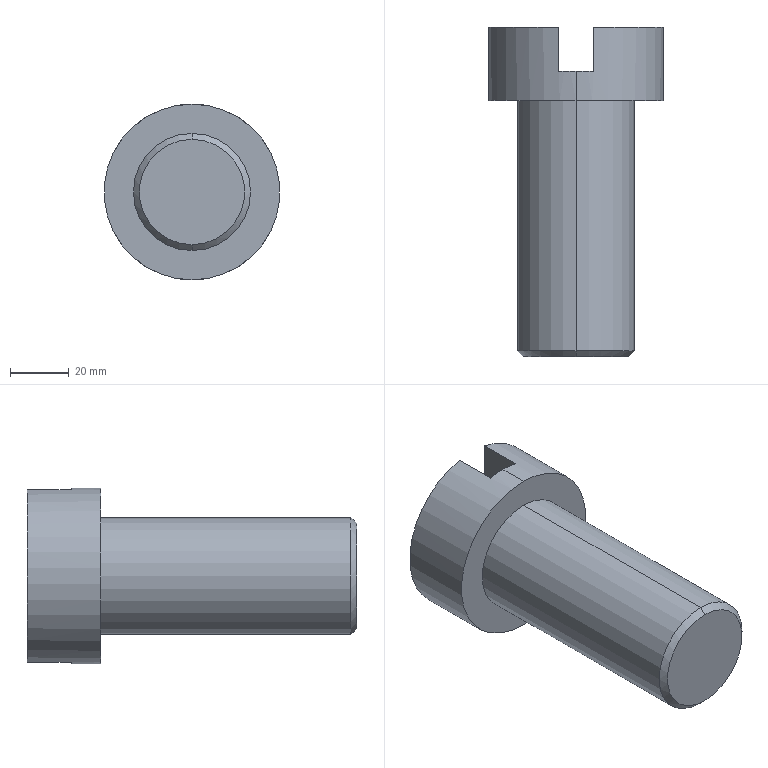Part | SolidWorks | features ICE 2, Chamfer 1, Extrusion 1 | 1 solid | 13 faces | box 60 x 112.5 x 60 mm | volume 169671 mm3 | plane 7 | cylinder 4 | cone 2 | commonest cylinder face diameters 40 x2 60 x2
STEP:
#1=CARTESIAN_POINT('',(0.,-50.,-18.));
#2=VERTEX_POINT('',#1);
#3=CARTESIAN_POINT('',(0.,-50.,18.));
#4=VERTEX_POINT('',#3);
#5=CARTESIAN_POINT('',(0.,-50.,0.));
#6=DIRECTION('',(0.,-1.,0.));
#7=DIRECTION('',(0.,0.,1.));
#8=AXIS2_PLACEMENT_3D('',#5,#6,#7);
#9=CIRCLE('',#8,18.);
#10=EDGE_CURVE('',#2,#4,#9,.T.);
#11=ORIENTED_EDGE('',*,*,#10,.F.);
#12=CARTESIAN_POINT('',(0.,-48.,-20.));
#13=VERTEX_POINT('',#12);
#14=CARTESIAN_POINT('',(0.,-48.,-20.));
#15=DIRECTION('',(0.,0.7071,-0.7071));
#16=VECTOR('',#15,1000.);
#17=LINE('',#14,#16);
#18=EDGE_CURVE('',#2,#13,#17,.T.);
#19=ORIENTED_EDGE('',*,*,#18,.T.);
#20=CARTESIAN_POINT('',(0.,-48.,20.));
#21=VERTEX_POINT('',#20);
#22=CARTESIAN_POINT('',(0.,-48.,0.));
#23=DIRECTION('',(0.,1.,0.));
#24=DIRECTION('',(0.,0.,1.));
#25=AXIS2_PLACEMENT_3D('',#22,#23,#24);
#26=CIRCLE('',#25,20.);
#27=EDGE_CURVE('',#21,#13,#26,.T.);
#28=ORIENTED_EDGE('',*,*,#27,.F.);
#29=CARTESIAN_POINT('',(0.,-48.,20.));
#30=DIRECTION('',(0.,0.7071,0.7071));
#31=VECTOR('',#30,1000.);
#32=LINE('',#29,#31);
#33=EDGE_CURVE('',#4,#21,#32,.T.);
#34=ORIENTED_EDGE('',*,*,#33,.F.);
#35=EDGE_LOOP('',(#11,#19,#28,#34));
#36=FACE_OUTER_BOUND('',#35,.T.);
#37=CARTESIAN_POINT('',(0.,-48.,0.));
#38=DIRECTION('',(0.,1.,0.));
#39=DIRECTION('',(0.,0.,1.));
#40=AXIS2_PLACEMENT_3D('',#37,#38,#39);
#41=CONICAL_SURFACE('',#40,20.,0.7854);
#42=ADVANCED_FACE('',(#36),#41,.T.);
#43=CARTESIAN_POINT('',(0.,37.5,20.));
#44=VERTEX_POINT('',#43);
#45=CARTESIAN_POINT('',(0.,37.5,-20.));
#46=VERTEX_POINT('',#45);
#47=CARTESIAN_POINT('',(0.,37.5,0.));
#48=DIRECTION('',(0.,1.,0.));
#49=DIRECTION('',(0.,0.,1.));
#50=AXIS2_PLACEMENT_3D('',#47,#48,#49);
#51=CIRCLE('',#50,20.);
#52=EDGE_CURVE('',#44,#46,#51,.T.);
#53=ORIENTED_EDGE('',*,*,#52,.F.);
#54=CARTESIAN_POINT('',(0.,50.,20.));
#55=DIRECTION('',(0.,-1.,0.));
#56=VECTOR('',#55,1000.);
#57=LINE('',#54,#56);
#58=EDGE_CURVE('',#44,#21,#57,.T.);
#59=ORIENTED_EDGE('',*,*,#58,.T.);
#60=ORIENTED_EDGE('',*,*,#27,.T.);
#61=CARTESIAN_POINT('',(0.,50.,-20.));
#62=DIRECTION('',(0.,-1.,0.));
#63=VECTOR('',#62,1000.);
#64=LINE('',#61,#63);
#65=EDGE_CURVE('',#46,#13,#64,.T.);
#66=ORIENTED_EDGE('',*,*,#65,.F.);
#67=EDGE_LOOP('',(#53,#59,#60,#66));
#68=FACE_OUTER_BOUND('',#67,.T.);
#69=CARTESIAN_POINT('',(0.,50.,0.));
#70=DIRECTION('',(0.,-1.,0.));
#71=DIRECTION('',(0.,0.,-1.));
#72=AXIS2_PLACEMENT_3D('',#69,#70,#71);
#73=CYLINDRICAL_SURFACE('',#72,20.);
#74=ADVANCED_FACE('',(#68),#73,.T.);
#75=CARTESIAN_POINT('',(0.,47.5,30.));
#76=VERTEX_POINT('',#75);
#77=CARTESIAN_POINT('',(6.,47.5,29.394));
#78=VERTEX_POINT('',#77);
#79=CARTESIAN_POINT('',(0.,47.5,0.));
#80=DIRECTION('',(0.,1.,0.));
#81=DIRECTION('',(0.,0.,1.));
#82=AXIS2_PLACEMENT_3D('',#79,#80,#81);
#83=CIRCLE('',#82,30.);
#84=EDGE_CURVE('',#76,#78,#83,.T.);
#85=ORIENTED_EDGE('',*,*,#84,.F.);
#86=CARTESIAN_POINT('',(0.,37.5,30.));
#87=VERTEX_POINT('',#86);
#88=CARTESIAN_POINT('',(0.,62.5,30.));
#89=DIRECTION('',(0.,-1.,0.));
#90=VECTOR('',#89,1000.);
#91=LINE('',#88,#90);
#92=EDGE_CURVE('',#76,#87,#91,.T.);
#93=ORIENTED_EDGE('',*,*,#92,.T.);
#94=CARTESIAN_POINT('',(0.,37.5,-30.));
#95=VERTEX_POINT('',#94);
#96=CARTESIAN_POINT('',(0.,37.5,0.));
#97=DIRECTION('',(0.,1.,0.));
#98=DIRECTION('',(0.,0.,1.));
#99=AXIS2_PLACEMENT_3D('',#96,#97,#98);
#100=CIRCLE('',#99,30.);
#101=EDGE_CURVE('',#87,#95,#100,.T.);
#102=ORIENTED_EDGE('',*,*,#101,.T.);
#103=CARTESIAN_POINT('',(0.,47.5,-30.));
#104=VERTEX_POINT('',#103);
#105=CARTESIAN_POINT('',(0.,62.5,-30.));
#106=DIRECTION('',(0.,-1.,0.));
#107=VECTOR('',#106,1000.);
#108=LINE('',#105,#107);
#109=EDGE_CURVE('',#104,#95,#108,.T.);
#110=ORIENTED_EDGE('',*,*,#109,.F.);
#111=CARTESIAN_POINT('',(6.,47.5,-29.394));
#112=VERTEX_POINT('',#111);
#113=CARTESIAN_POINT('',(0.,47.5,0.));
#114=DIRECTION('',(0.,1.,0.));
#115=DIRECTION('',(0.,0.,1.));
#116=AXIS2_PLACEMENT_3D('',#113,#114,#115);
#117=CIRCLE('',#116,30.);
#118=EDGE_CURVE('',#112,#104,#117,.T.);
#119=ORIENTED_EDGE('',*,*,#118,.F.);
#120=CARTESIAN_POINT('',(6.,62.5,-29.394));
#121=VERTEX_POINT('',#120);
#122=CARTESIAN_POINT('',(6.,62.5,-29.394));
#123=DIRECTION('',(0.,1.,0.));
#124=VECTOR('',#123,1000.);
#125=LINE('',#122,#124);
#126=EDGE_CURVE('',#112,#121,#125,.T.);
#127=ORIENTED_EDGE('',*,*,#126,.T.);
#128=CARTESIAN_POINT('',(6.,62.5,29.394));
#129=VERTEX_POINT('',#128);
#130=CARTESIAN_POINT('',(0.,62.5,0.));
#131=DIRECTION('',(0.,1.,0.));
#132=DIRECTION('',(0.,0.,1.));
#133=AXIS2_PLACEMENT_3D('',#130,#131,#132);
#134=CIRCLE('',#133,30.);
#135=EDGE_CURVE('',#129,#121,#134,.T.);
#136=ORIENTED_EDGE('',*,*,#135,.F.);
#137=CARTESIAN_POINT('',(6.,62.5,29.394));
#138=DIRECTION('',(0.,-1.,0.));
#139=VECTOR('',#138,1000.);
#140=LINE('',#137,#139);
#141=EDGE_CURVE('',#129,#78,#140,.T.);
#142=ORIENTED_EDGE('',*,*,#141,.T.);
#143=EDGE_LOOP('',(#85,#93,#102,#110,#119,#127,#136,#142));
#144=FACE_OUTER_BOUND('',#143,.T.);
#145=CARTESIAN_POINT('',(0.,62.5,0.));
#146=DIRECTION('',(0.,-1.,0.));
#147=DIRECTION('',(0.,0.,-1.));
#148=AXIS2_PLACEMENT_3D('',#145,#146,#147);
#149=CYLINDRICAL_SURFACE('',#148,30.);
#150=ADVANCED_FACE('',(#144),#149,.T.);
#151=ORIENTED_EDGE('',*,*,#92,.F.);
#152=CARTESIAN_POINT('',(-6.,47.5,29.394));
#153=VERTEX_POINT('',#152);
#154=CARTESIAN_POINT('',(0.,47.5,0.));
#155=DIRECTION('',(0.,1.,0.));
#156=DIRECTION('',(0.,0.,1.));
#157=AXIS2_PLACEMENT_3D('',#154,#155,#156);
#158=CIRCLE('',#157,30.);
#159=EDGE_CURVE('',#153,#76,#158,.T.);
#160=ORIENTED_EDGE('',*,*,#159,.F.);
#161=CARTESIAN_POINT('',(-6.,62.5,29.394));
#162=VERTEX_POINT('',#161);
#163=CARTESIAN_POINT('',(-6.,62.5,29.394));
#164=DIRECTION('',(0.,-1.,0.));
#165=VECTOR('',#164,1000.);
#166=LINE('',#163,#165);
#167=EDGE_CURVE('',#162,#153,#166,.T.);
#168=ORIENTED_EDGE('',*,*,#167,.F.);
#169=CARTESIAN_POINT('',(-6.,62.5,-29.394));
#170=VERTEX_POINT('',#169);
#171=CARTESIAN_POINT('',(0.,62.5,0.));
#172=DIRECTION('',(0.,1.,0.));
#173=DIRECTION('',(0.,0.,1.));
#174=AXIS2_PLACEMENT_3D('',#171,#172,#173);
#175=CIRCLE('',#174,30.);
#176=EDGE_CURVE('',#170,#162,#175,.T.);
#177=ORIENTED_EDGE('',*,*,#176,.F.);
#178=CARTESIAN_POINT('',(-6.,47.5,-29.394));
#179=VERTEX_POINT('',#178);
#180=CARTESIAN_POINT('',(-6.,62.5,-29.394));
#181=DIRECTION('',(0.,1.,0.));
#182=VECTOR('',#181,1000.);
#183=LINE('',#180,#182);
#184=EDGE_CURVE('',#179,#170,#183,.T.);
#185=ORIENTED_EDGE('',*,*,#184,.F.);
#186=CARTESIAN_POINT('',(0.,47.5,0.));
#187=DIRECTION('',(0.,1.,0.));
#188=DIRECTION('',(0.,0.,1.));
#189=AXIS2_PLACEMENT_3D('',#186,#187,#188);
#190=CIRCLE('',#189,30.);
#191=EDGE_CURVE('',#104,#179,#190,.T.);
#192=ORIENTED_EDGE('',*,*,#191,.F.);
#193=ORIENTED_EDGE('',*,*,#109,.T.);
#194=CARTESIAN_POINT('',(0.,37.5,0.));
#195=DIRECTION('',(0.,1.,0.));
#196=DIRECTION('',(0.,0.,1.));
#197=AXIS2_PLACEMENT_3D('',#194,#195,#196);
#198=CIRCLE('',#197,30.);
#199=EDGE_CURVE('',#95,#87,#198,.T.);
#200=ORIENTED_EDGE('',*,*,#199,.T.);
#201=EDGE_LOOP('',(#151,#160,#168,#177,#185,#192,#193,#200));
#202=FACE_OUTER_BOUND('',#201,.T.);
#203=CARTESIAN_POINT('',(0.,62.5,0.));
#204=DIRECTION('',(0.,-1.,0.));
#205=DIRECTION('',(0.,0.,-1.));
#206=AXIS2_PLACEMENT_3D('',#203,#204,#205);
#207=CYLINDRICAL_SURFACE('',#206,30.);
#208=ADVANCED_FACE('',(#202),#207,.T.);
#209=ORIENTED_EDGE('',*,*,#176,.T.);
#210=CARTESIAN_POINT('',(-6.,62.5,0.));
#211=DIRECTION('',(0.,0.,-1.));
#212=VECTOR('',#211,1000.);
#213=LINE('',#210,#212);
#214=EDGE_CURVE('',#162,#170,#213,.T.);
#215=ORIENTED_EDGE('',*,*,#214,.T.);
#216=EDGE_LOOP('',(#209,#215));
#217=FACE_OUTER_BOUND('',#216,.T.);
#218=CARTESIAN_POINT('',(0.,62.5,0.));
#219=DIRECTION('',(0.,1.,0.));
#220=DIRECTION('',(0.,0.,1.));
#221=AXIS2_PLACEMENT_3D('',#218,#219,#220);
#222=PLANE('',#221);
#223=ADVANCED_FACE('',(#217),#222,.T.);
#224=ORIENTED_EDGE('',*,*,#58,.F.);
#225=CARTESIAN_POINT('',(0.,37.5,0.));
#226=DIRECTION('',(0.,1.,0.));
#227=DIRECTION('',(0.,0.,1.));
#228=AXIS2_PLACEMENT_3D('',#225,#226,#227);
#229=CIRCLE('',#228,20.);
#230=EDGE_CURVE('',#46,#44,#229,.T.);
#231=ORIENTED_EDGE('',*,*,#230,.F.);
#232=ORIENTED_EDGE('',*,*,#65,.T.);
#233=CARTESIAN_POINT('',(0.,-48.,0.));
#234=DIRECTION('',(0.,1.,0.));
#235=DIRECTION('',(0.,0.,1.));
#236=AXIS2_PLACEMENT_3D('',#233,#234,#235);
#237=CIRCLE('',#236,20.);
#238=EDGE_CURVE('',#13,#21,#237,.T.);
#239=ORIENTED_EDGE('',*,*,#238,.T.);
#240=EDGE_LOOP('',(#224,#231,#232,#239));
#241=FACE_OUTER_BOUND('',#240,.T.);
#242=CARTESIAN_POINT('',(0.,50.,0.));
#243=DIRECTION('',(0.,-1.,0.));
#244=DIRECTION('',(0.,0.,-1.));
#245=AXIS2_PLACEMENT_3D('',#242,#243,#244);
#246=CYLINDRICAL_SURFACE('',#245,20.);
#247=ADVANCED_FACE('',(#241),#246,.T.);
#248=CARTESIAN_POINT('',(0.,-50.,0.));
#249=DIRECTION('',(0.,-1.,0.));
#250=DIRECTION('',(0.,0.,1.));
#251=AXIS2_PLACEMENT_3D('',#248,#249,#250);
#252=CIRCLE('',#251,18.);
#253=EDGE_CURVE('',#4,#2,#252,.T.);
#254=ORIENTED_EDGE('',*,*,#253,.T.);
#255=ORIENTED_EDGE('',*,*,#10,.T.);
#256=EDGE_LOOP('',(#254,#255));
#257=FACE_OUTER_BOUND('',#256,.T.);
#258=CARTESIAN_POINT('',(0.,-50.,0.));
#259=DIRECTION('',(0.,1.,0.));
#260=DIRECTION('',(0.,0.,1.));
#261=AXIS2_PLACEMENT_3D('',#258,#259,#260);
#262=PLANE('',#261);
#263=ADVANCED_FACE('',(#257),#262,.F.);
#264=CARTESIAN_POINT('',(6.,62.5,0.));
#265=DIRECTION('',(0.,0.,-1.));
#266=VECTOR('',#265,1000.);
#267=LINE('',#264,#266);
#268=EDGE_CURVE('',#129,#121,#267,.T.);
#269=ORIENTED_EDGE('',*,*,#268,.F.);
#270=ORIENTED_EDGE('',*,*,#135,.T.);
#271=EDGE_LOOP('',(#269,#270));
#272=FACE_OUTER_BOUND('',#271,.T.);
#273=CARTESIAN_POINT('',(0.,62.5,0.));
#274=DIRECTION('',(0.,1.,0.));
#275=DIRECTION('',(0.,0.,1.));
#276=AXIS2_PLACEMENT_3D('',#273,#274,#275);
#277=PLANE('',#276);
#278=ADVANCED_FACE('',(#272),#277,.T.);
#279=ORIENTED_EDGE('',*,*,#230,.T.);
#280=ORIENTED_EDGE('',*,*,#52,.T.);
#281=EDGE_LOOP('',(#279,#280));
#282=FACE_BOUND('',#281,.T.);
#283=ORIENTED_EDGE('',*,*,#199,.F.);
#284=ORIENTED_EDGE('',*,*,#101,.F.);
#285=EDGE_LOOP('',(#283,#284));
#286=FACE_OUTER_BOUND('',#285,.T.);
#287=CARTESIAN_POINT('',(0.,37.5,0.));
#288=DIRECTION('',(0.,1.,0.));
#289=DIRECTION('',(0.,0.,1.));
#290=AXIS2_PLACEMENT_3D('',#287,#288,#289);
#291=PLANE('',#290);
#292=ADVANCED_FACE('',(#282,#286),#291,.F.);
#293=ORIENTED_EDGE('',*,*,#18,.F.);
#294=ORIENTED_EDGE('',*,*,#253,.F.);
#295=ORIENTED_EDGE('',*,*,#33,.T.);
#296=ORIENTED_EDGE('',*,*,#238,.F.);
#297=EDGE_LOOP('',(#293,#294,#295,#296));
#298=FACE_OUTER_BOUND('',#297,.T.);
#299=CARTESIAN_POINT('',(0.,-48.,0.));
#300=DIRECTION('',(0.,1.,0.));
#301=DIRECTION('',(0.,0.,1.));
#302=AXIS2_PLACEMENT_3D('',#299,#300,#301);
#303=CONICAL_SURFACE('',#302,20.,0.7854);
#304=ADVANCED_FACE('',(#298),#303,.T.);
#305=ORIENTED_EDGE('',*,*,#118,.T.);
#306=ORIENTED_EDGE('',*,*,#191,.T.);
#307=CARTESIAN_POINT('',(-6.,47.5,38.749));
#308=DIRECTION('',(0.,0.,-1.));
#309=VECTOR('',#308,1000.);
#310=LINE('',#307,#309);
#311=EDGE_CURVE('',#153,#179,#310,.T.);
#312=ORIENTED_EDGE('',*,*,#311,.F.);
#313=ORIENTED_EDGE('',*,*,#159,.T.);
#314=ORIENTED_EDGE('',*,*,#84,.T.);
#315=CARTESIAN_POINT('',(6.,47.5,38.749));
#316=DIRECTION('',(0.,0.,-1.));
#317=VECTOR('',#316,1000.);
#318=LINE('',#315,#317);
#319=EDGE_CURVE('',#78,#112,#318,.T.);
#320=ORIENTED_EDGE('',*,*,#319,.T.);
#321=EDGE_LOOP('',(#305,#306,#312,#313,#314,#320));
#322=FACE_OUTER_BOUND('',#321,.T.);
#323=CARTESIAN_POINT('',(0.,47.5,0.));
#324=DIRECTION('',(0.,1.,0.));
#325=DIRECTION('',(0.,0.,1.));
#326=AXIS2_PLACEMENT_3D('',#323,#324,#325);
#327=PLANE('',#326);
#328=ADVANCED_FACE('',(#322),#327,.T.);
#329=ORIENTED_EDGE('',*,*,#167,.T.);
#330=ORIENTED_EDGE('',*,*,#311,.T.);
#331=ORIENTED_EDGE('',*,*,#184,.T.);
#332=ORIENTED_EDGE('',*,*,#214,.F.);
#333=EDGE_LOOP('',(#329,#330,#331,#332));
#334=FACE_OUTER_BOUND('',#333,.T.);
#335=CARTESIAN_POINT('',(-6.,47.5,38.749));
#336=DIRECTION('',(1.,0.,0.));
#337=DIRECTION('',(0.,0.,-1.));
#338=AXIS2_PLACEMENT_3D('',#335,#336,#337);
#339=PLANE('',#338);
#340=ADVANCED_FACE('',(#334),#339,.T.);
#341=ORIENTED_EDGE('',*,*,#268,.T.);
#342=ORIENTED_EDGE('',*,*,#126,.F.);
#343=ORIENTED_EDGE('',*,*,#319,.F.);
#344=ORIENTED_EDGE('',*,*,#141,.F.);
#345=EDGE_LOOP('',(#341,#342,#343,#344));
#346=FACE_OUTER_BOUND('',#345,.T.);
#347=CARTESIAN_POINT('',(6.,47.5,38.749));
#348=DIRECTION('',(1.,0.,0.));
#349=DIRECTION('',(0.,0.,-1.));
#350=AXIS2_PLACEMENT_3D('',#347,#348,#349);
#351=PLANE('',#350);
#352=ADVANCED_FACE('',(#346),#351,.F.);
#353=CLOSED_SHELL('',(#42,#74,#150,#208,#223,#247,#263,#278,#292,#304,#328,#340,#352));
#354=MANIFOLD_SOLID_BREP('',#353);
#355=CARTESIAN_POINT('',(0.,0.,0.));
#356=DIRECTION('',(0.,0.,1.));
#357=DIRECTION('',(1.,0.,0.));
#358=AXIS2_PLACEMENT_3D('',#355,#356,#357);
#359=(LENGTH_UNIT()NAMED_UNIT(*)SI_UNIT(.MILLI.,.METRE.));
#360=UNCERTAINTY_MEASURE_WITH_UNIT(LENGTH_MEASURE(0.00001),#359,'','');
#361=(NAMED_UNIT(*)PLANE_ANGLE_UNIT()SI_UNIT($,.RADIAN.));
#362=(NAMED_UNIT(*)SI_UNIT($,.STERADIAN.)SOLID_ANGLE_UNIT());
#363=(GEOMETRIC_REPRESENTATION_CONTEXT(3)GLOBAL_UNCERTAINTY_ASSIGNED_CONTEXT((#360))GLOBAL_UNIT_ASSIGNED_CONTEXT((#359,#361,#362))REPRESENTATION_CONTEXT('',''));
#364=ADVANCED_BREP_SHAPE_REPRESENTATION('',(#354,#358),#363);